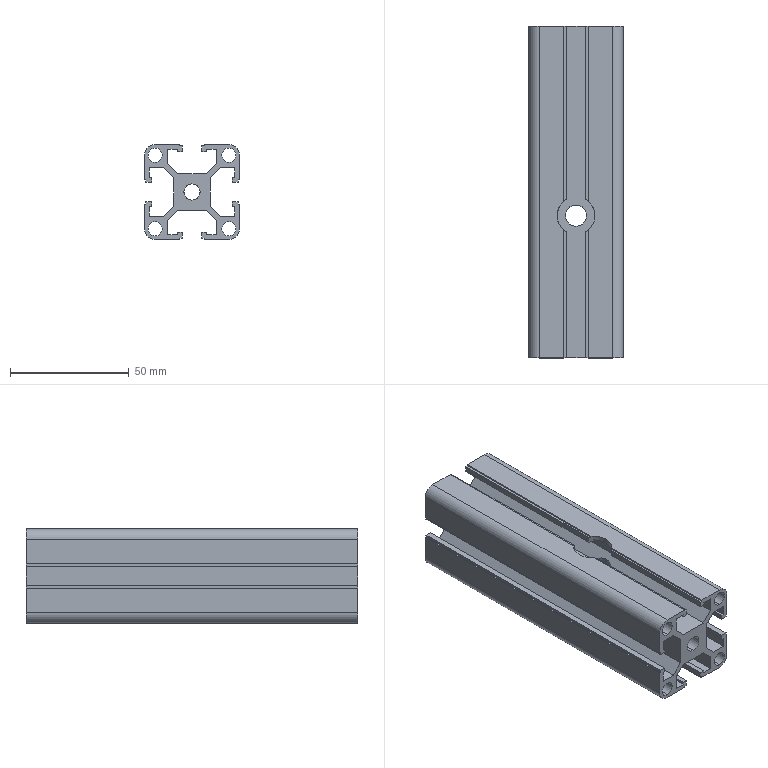Part | SolidWorks | features HoleWzd 1, WeldMemberFeat 1, WeldmentFeature 1 | 1 solid | 117 faces | box 40 x 140 x 40 mm | volume 83784 mm3 | plane 90 | cylinder 27 | commonest cylinder face diameters 9 x9 6 x8 16 x6 6.8 x4